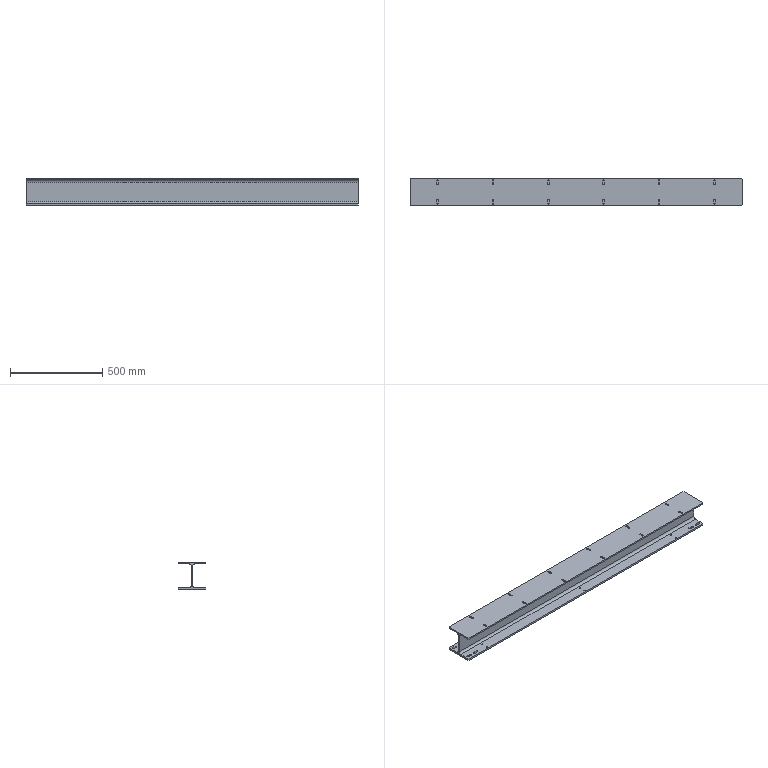Part | NX | features BREP 1 | 1 solid | 126 faces | box 1800 x 150 x 148 mm | volume 6711665 mm3 | cylinder 64 | plane 62 | commonest cylinder face diameters 9 x24 11 x24 7 x12 26 x4